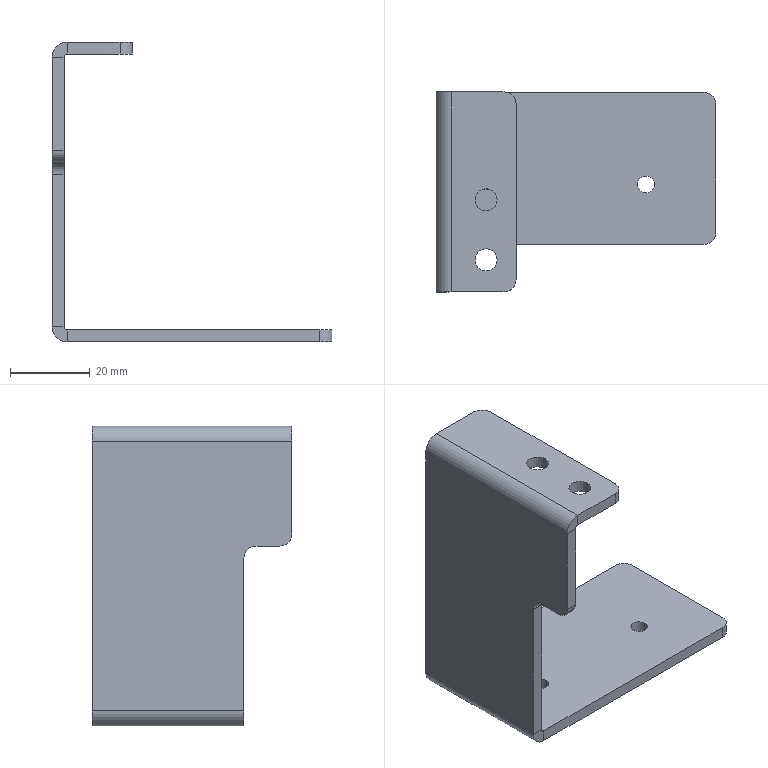Part | SolidWorks | features Fillet 2, HoleWzd 2, FlatPattern 1, ICE 1, SMBaseFlange 1, SheetMetal 1 | 1 solid | 38 faces | box 70 x 50 x 75 mm | volume 19314 mm3 | plane 20 | cylinder 18 | commonest cylinder face diameters 6 x6 4.2 x4 5.5 x4 1.5 x2 7.5 x2
STEP:
#1=CARTESIAN_POINT('',(54.6,27.,-72.));
#2=VERTEX_POINT('',#1);
#3=CARTESIAN_POINT('',(50.4,27.,-72.));
#4=VERTEX_POINT('',#3);
#5=CARTESIAN_POINT('',(52.5,27.,-72.));
#6=DIRECTION('',(0.,0.,-1.));
#7=DIRECTION('',(-1.,0.,0.));
#8=AXIS2_PLACEMENT_3D('',#5,#6,#7);
#9=CIRCLE('',#8,2.1);
#10=EDGE_CURVE('',#2,#4,#9,.T.);
#11=ORIENTED_EDGE('',*,*,#10,.F.);
#12=CARTESIAN_POINT('',(54.6,27.,-75.));
#13=VERTEX_POINT('',#12);
#14=CARTESIAN_POINT('',(54.6,27.,-75.));
#15=DIRECTION('',(0.,0.,-1.));
#16=VECTOR('',#15,1000.);
#17=LINE('',#14,#16);
#18=EDGE_CURVE('',#2,#13,#17,.T.);
#19=ORIENTED_EDGE('',*,*,#18,.T.);
#20=CARTESIAN_POINT('',(50.4,27.,-75.));
#21=VERTEX_POINT('',#20);
#22=CARTESIAN_POINT('',(52.5,27.,-75.));
#23=DIRECTION('',(0.,0.,-1.));
#24=DIRECTION('',(-1.,0.,0.));
#25=AXIS2_PLACEMENT_3D('',#22,#23,#24);
#26=CIRCLE('',#25,2.1);
#27=EDGE_CURVE('',#13,#21,#26,.T.);
#28=ORIENTED_EDGE('',*,*,#27,.T.);
#29=CARTESIAN_POINT('',(50.4,27.,-75.));
#30=DIRECTION('',(0.,0.,-1.));
#31=VECTOR('',#30,1000.);
#32=LINE('',#29,#31);
#33=EDGE_CURVE('',#4,#21,#32,.T.);
#34=ORIENTED_EDGE('',*,*,#33,.F.);
#35=EDGE_LOOP('',(#11,#19,#28,#34));
#36=FACE_OUTER_BOUND('',#35,.T.);
#37=CARTESIAN_POINT('',(52.5,27.,-75.));
#38=DIRECTION('',(0.,0.,-1.));
#39=DIRECTION('',(-1.,0.,0.));
#40=AXIS2_PLACEMENT_3D('',#37,#38,#39);
#41=CYLINDRICAL_SURFACE('',#40,2.1);
#42=ADVANCED_FACE('',(#36),#41,.F.);
#43=CARTESIAN_POINT('',(19.6,27.,-72.));
#44=VERTEX_POINT('',#43);
#45=CARTESIAN_POINT('',(15.4,27.,-72.));
#46=VERTEX_POINT('',#45);
#47=CARTESIAN_POINT('',(17.5,27.,-72.));
#48=DIRECTION('',(0.,0.,-1.));
#49=DIRECTION('',(-1.,0.,0.));
#50=AXIS2_PLACEMENT_3D('',#47,#48,#49);
#51=CIRCLE('',#50,2.1);
#52=EDGE_CURVE('',#44,#46,#51,.T.);
#53=ORIENTED_EDGE('',*,*,#52,.F.);
#54=CARTESIAN_POINT('',(19.6,27.,-75.));
#55=VERTEX_POINT('',#54);
#56=CARTESIAN_POINT('',(19.6,27.,-75.));
#57=DIRECTION('',(0.,0.,-1.));
#58=VECTOR('',#57,1000.);
#59=LINE('',#56,#58);
#60=EDGE_CURVE('',#44,#55,#59,.T.);
#61=ORIENTED_EDGE('',*,*,#60,.T.);
#62=CARTESIAN_POINT('',(15.4,27.,-75.));
#63=VERTEX_POINT('',#62);
#64=CARTESIAN_POINT('',(17.5,27.,-75.));
#65=DIRECTION('',(0.,0.,-1.));
#66=DIRECTION('',(-1.,0.,0.));
#67=AXIS2_PLACEMENT_3D('',#64,#65,#66);
#68=CIRCLE('',#67,2.1);
#69=EDGE_CURVE('',#55,#63,#68,.T.);
#70=ORIENTED_EDGE('',*,*,#69,.T.);
#71=CARTESIAN_POINT('',(15.4,27.,-75.));
#72=DIRECTION('',(0.,0.,-1.));
#73=VECTOR('',#72,1000.);
#74=LINE('',#71,#73);
#75=EDGE_CURVE('',#46,#63,#74,.T.);
#76=ORIENTED_EDGE('',*,*,#75,.F.);
#77=EDGE_LOOP('',(#53,#61,#70,#76));
#78=FACE_OUTER_BOUND('',#77,.T.);
#79=CARTESIAN_POINT('',(17.5,27.,-75.));
#80=DIRECTION('',(0.,0.,-1.));
#81=DIRECTION('',(-1.,0.,0.));
#82=AXIS2_PLACEMENT_3D('',#79,#80,#81);
#83=CYLINDRICAL_SURFACE('',#82,2.1);
#84=ADVANCED_FACE('',(#78),#83,.F.);
#85=CARTESIAN_POINT('',(9.75,23.,-3.));
#86=VERTEX_POINT('',#85);
#87=CARTESIAN_POINT('',(15.25,23.,-3.));
#88=VERTEX_POINT('',#87);
#89=CARTESIAN_POINT('',(12.5,23.,-3.));
#90=DIRECTION('',(0.,0.,1.));
#91=DIRECTION('',(1.,0.,0.));
#92=AXIS2_PLACEMENT_3D('',#89,#90,#91);
#93=CIRCLE('',#92,2.75);
#94=EDGE_CURVE('',#86,#88,#93,.T.);
#95=ORIENTED_EDGE('',*,*,#94,.F.);
#96=CARTESIAN_POINT('',(9.75,23.,0.));
#97=VERTEX_POINT('',#96);
#98=CARTESIAN_POINT('',(9.75,23.,0.));
#99=DIRECTION('',(0.,0.,1.));
#100=VECTOR('',#99,1000.);
#101=LINE('',#98,#100);
#102=EDGE_CURVE('',#86,#97,#101,.T.);
#103=ORIENTED_EDGE('',*,*,#102,.T.);
#104=CARTESIAN_POINT('',(15.25,23.,0.));
#105=VERTEX_POINT('',#104);
#106=CARTESIAN_POINT('',(12.5,23.,0.));
#107=DIRECTION('',(0.,0.,1.));
#108=DIRECTION('',(1.,0.,0.));
#109=AXIS2_PLACEMENT_3D('',#106,#107,#108);
#110=CIRCLE('',#109,2.75);
#111=EDGE_CURVE('',#97,#105,#110,.T.);
#112=ORIENTED_EDGE('',*,*,#111,.T.);
#113=CARTESIAN_POINT('',(15.25,23.,0.));
#114=DIRECTION('',(0.,0.,1.));
#115=VECTOR('',#114,1000.);
#116=LINE('',#113,#115);
#117=EDGE_CURVE('',#88,#105,#116,.T.);
#118=ORIENTED_EDGE('',*,*,#117,.F.);
#119=EDGE_LOOP('',(#95,#103,#112,#118));
#120=FACE_OUTER_BOUND('',#119,.T.);
#121=CARTESIAN_POINT('',(12.5,23.,0.));
#122=DIRECTION('',(0.,0.,1.));
#123=DIRECTION('',(1.,0.,0.));
#124=AXIS2_PLACEMENT_3D('',#121,#122,#123);
#125=CYLINDRICAL_SURFACE('',#124,2.75);
#126=ADVANCED_FACE('',(#120),#125,.F.);
#127=CARTESIAN_POINT('',(9.75,8.,-3.));
#128=VERTEX_POINT('',#127);
#129=CARTESIAN_POINT('',(15.25,8.,-3.));
#130=VERTEX_POINT('',#129);
#131=CARTESIAN_POINT('',(12.5,8.,-3.));
#132=DIRECTION('',(0.,0.,1.));
#133=DIRECTION('',(1.,0.,0.));
#134=AXIS2_PLACEMENT_3D('',#131,#132,#133);
#135=CIRCLE('',#134,2.75);
#136=EDGE_CURVE('',#128,#130,#135,.T.);
#137=ORIENTED_EDGE('',*,*,#136,.F.);
#138=CARTESIAN_POINT('',(9.75,8.,0.));
#139=VERTEX_POINT('',#138);
#140=CARTESIAN_POINT('',(9.75,8.,0.));
#141=DIRECTION('',(0.,0.,1.));
#142=VECTOR('',#141,1000.);
#143=LINE('',#140,#142);
#144=EDGE_CURVE('',#128,#139,#143,.T.);
#145=ORIENTED_EDGE('',*,*,#144,.T.);
#146=CARTESIAN_POINT('',(15.25,8.,0.));
#147=VERTEX_POINT('',#146);
#148=CARTESIAN_POINT('',(12.5,8.,0.));
#149=DIRECTION('',(0.,0.,1.));
#150=DIRECTION('',(1.,0.,0.));
#151=AXIS2_PLACEMENT_3D('',#148,#149,#150);
#152=CIRCLE('',#151,2.75);
#153=EDGE_CURVE('',#139,#147,#152,.T.);
#154=ORIENTED_EDGE('',*,*,#153,.T.);
#155=CARTESIAN_POINT('',(15.25,8.,0.));
#156=DIRECTION('',(0.,0.,1.));
#157=VECTOR('',#156,1000.);
#158=LINE('',#155,#157);
#159=EDGE_CURVE('',#130,#147,#158,.T.);
#160=ORIENTED_EDGE('',*,*,#159,.F.);
#161=EDGE_LOOP('',(#137,#145,#154,#160));
#162=FACE_OUTER_BOUND('',#161,.T.);
#163=CARTESIAN_POINT('',(12.5,8.,0.));
#164=DIRECTION('',(0.,0.,1.));
#165=DIRECTION('',(1.,0.,0.));
#166=AXIS2_PLACEMENT_3D('',#163,#164,#165);
#167=CYLINDRICAL_SURFACE('',#166,2.75);
#168=ADVANCED_FACE('',(#162),#167,.F.);
#169=CARTESIAN_POINT('',(67.,12.,-75.));
#170=VERTEX_POINT('',#169);
#171=CARTESIAN_POINT('',(3.75,12.,-75.));
#172=VERTEX_POINT('',#171);
#173=CARTESIAN_POINT('',(70.,12.,-75.));
#174=DIRECTION('',(-1.,0.,0.));
#175=VECTOR('',#174,1000.);
#176=LINE('',#173,#175);
#177=EDGE_CURVE('',#170,#172,#176,.T.);
#178=ORIENTED_EDGE('',*,*,#177,.F.);
#179=CARTESIAN_POINT('',(67.,12.,-72.));
#180=VERTEX_POINT('',#179);
#181=CARTESIAN_POINT('',(67.,12.,-72.));
#182=DIRECTION('',(0.,0.,1.));
#183=VECTOR('',#182,1000.);
#184=LINE('',#181,#183);
#185=EDGE_CURVE('',#170,#180,#184,.T.);
#186=ORIENTED_EDGE('',*,*,#185,.T.);
#187=CARTESIAN_POINT('',(3.75,12.,-72.));
#188=VERTEX_POINT('',#187);
#189=CARTESIAN_POINT('',(0.,12.,-72.));
#190=DIRECTION('',(1.,0.,0.));
#191=VECTOR('',#190,1000.);
#192=LINE('',#189,#191);
#193=EDGE_CURVE('',#188,#180,#192,.T.);
#194=ORIENTED_EDGE('',*,*,#193,.F.);
#195=CARTESIAN_POINT('',(3.75,12.,-72.));
#196=DIRECTION('',(0.,0.,-1.));
#197=VECTOR('',#196,1000.);
#198=LINE('',#195,#197);
#199=EDGE_CURVE('',#188,#172,#198,.T.);
#200=ORIENTED_EDGE('',*,*,#199,.T.);
#201=EDGE_LOOP('',(#178,#186,#194,#200));
#202=FACE_OUTER_BOUND('',#201,.T.);
#203=CARTESIAN_POINT('',(70.,12.,-75.));
#204=DIRECTION('',(0.,1.,0.));
#205=DIRECTION('',(0.,0.,1.));
#206=AXIS2_PLACEMENT_3D('',#203,#204,#205);
#207=PLANE('',#206);
#208=ADVANCED_FACE('',(#202),#207,.F.);
#209=CARTESIAN_POINT('',(3.,12.,-33.));
#210=VERTEX_POINT('',#209);
#211=CARTESIAN_POINT('',(3.,12.,-71.25));
#212=VERTEX_POINT('',#211);
#213=CARTESIAN_POINT('',(3.,12.,0.));
#214=DIRECTION('',(0.,0.,-1.));
#215=VECTOR('',#214,1000.);
#216=LINE('',#213,#215);
#217=EDGE_CURVE('',#210,#212,#216,.T.);
#218=ORIENTED_EDGE('',*,*,#217,.F.);
#219=CARTESIAN_POINT('',(0.,12.,-33.));
#220=VERTEX_POINT('',#219);
#221=CARTESIAN_POINT('',(0.,12.,-33.));
#222=DIRECTION('',(-1.,0.,0.));
#223=VECTOR('',#222,1000.);
#224=LINE('',#221,#223);
#225=EDGE_CURVE('',#210,#220,#224,.T.);
#226=ORIENTED_EDGE('',*,*,#225,.T.);
#227=CARTESIAN_POINT('',(0.,12.,-71.25));
#228=VERTEX_POINT('',#227);
#229=CARTESIAN_POINT('',(0.,12.,-75.));
#230=DIRECTION('',(0.,0.,-1.));
#231=VECTOR('',#230,1000.);
#232=LINE('',#229,#231);
#233=EDGE_CURVE('',#220,#228,#232,.T.);
#234=ORIENTED_EDGE('',*,*,#233,.T.);
#235=CARTESIAN_POINT('',(0.,12.,-71.25));
#236=DIRECTION('',(1.,0.,0.));
#237=VECTOR('',#236,1000.);
#238=LINE('',#235,#237);
#239=EDGE_CURVE('',#228,#212,#238,.T.);
#240=ORIENTED_EDGE('',*,*,#239,.T.);
#241=EDGE_LOOP('',(#218,#226,#234,#240));
#242=FACE_OUTER_BOUND('',#241,.T.);
#243=CARTESIAN_POINT('',(70.,12.,-75.));
#244=DIRECTION('',(0.,1.,0.));
#245=DIRECTION('',(0.,0.,1.));
#246=AXIS2_PLACEMENT_3D('',#243,#244,#245);
#247=PLANE('',#246);
#248=ADVANCED_FACE('',(#242),#247,.F.);
#249=CARTESIAN_POINT('',(0.,50.,-3.75));
#250=VERTEX_POINT('',#249);
#251=CARTESIAN_POINT('',(3.,50.,-3.75));
#252=VERTEX_POINT('',#251);
#253=CARTESIAN_POINT('',(0.,50.,-3.75));
#254=DIRECTION('',(1.,0.,0.));
#255=VECTOR('',#254,1000.);
#256=LINE('',#253,#255);
#257=EDGE_CURVE('',#250,#252,#256,.T.);
#258=ORIENTED_EDGE('',*,*,#257,.F.);
#259=CARTESIAN_POINT('',(3.75,50.,0.));
#260=VERTEX_POINT('',#259);
#261=CARTESIAN_POINT('',(3.75,50.,-3.75));
#262=DIRECTION('',(0.,-1.,0.));
#263=DIRECTION('',(0.,0.,1.));
#264=AXIS2_PLACEMENT_3D('',#261,#262,#263);
#265=CIRCLE('',#264,3.75);
#266=EDGE_CURVE('',#260,#250,#265,.T.);
#267=ORIENTED_EDGE('',*,*,#266,.F.);
#268=CARTESIAN_POINT('',(3.75,50.,-3.));
#269=VERTEX_POINT('',#268);
#270=CARTESIAN_POINT('',(3.75,50.,-3.));
#271=DIRECTION('',(0.,0.,1.));
#272=VECTOR('',#271,1000.);
#273=LINE('',#270,#272);
#274=EDGE_CURVE('',#269,#260,#273,.T.);
#275=ORIENTED_EDGE('',*,*,#274,.F.);
#276=CARTESIAN_POINT('',(3.75,50.,-3.75));
#277=DIRECTION('',(0.,-1.,0.));
#278=DIRECTION('',(1.,0.,0.));
#279=AXIS2_PLACEMENT_3D('',#276,#277,#278);
#280=CIRCLE('',#279,0.75);
#281=EDGE_CURVE('',#269,#252,#280,.T.);
#282=ORIENTED_EDGE('',*,*,#281,.T.);
#283=EDGE_LOOP('',(#258,#267,#275,#282));
#284=FACE_OUTER_BOUND('',#283,.T.);
#285=CARTESIAN_POINT('',(0.,50.,-3.75));
#286=DIRECTION('',(0.,1.,0.));
#287=DIRECTION('',(0.,0.,1.));
#288=AXIS2_PLACEMENT_3D('',#285,#286,#287);
#289=PLANE('',#288);
#290=ADVANCED_FACE('',(#284),#289,.T.);
#291=CARTESIAN_POINT('',(0.,50.,-71.25));
#292=VERTEX_POINT('',#291);
#293=CARTESIAN_POINT('',(0.,50.,0.));
#294=DIRECTION('',(0.,0.,-1.));
#295=VECTOR('',#294,1000.);
#296=LINE('',#293,#295);
#297=EDGE_CURVE('',#250,#292,#296,.T.);
#298=ORIENTED_EDGE('',*,*,#297,.F.);
#299=ORIENTED_EDGE('',*,*,#257,.T.);
#300=CARTESIAN_POINT('',(3.,50.,-71.25));
#301=VERTEX_POINT('',#300);
#302=CARTESIAN_POINT('',(3.,50.,0.));
#303=DIRECTION('',(0.,0.,-1.));
#304=VECTOR('',#303,1000.);
#305=LINE('',#302,#304);
#306=EDGE_CURVE('',#252,#301,#305,.T.);
#307=ORIENTED_EDGE('',*,*,#306,.T.);
#308=CARTESIAN_POINT('',(3.,50.,-71.25));
#309=DIRECTION('',(-1.,0.,0.));
#310=VECTOR('',#309,1000.);
#311=LINE('',#308,#310);
#312=EDGE_CURVE('',#301,#292,#311,.T.);
#313=ORIENTED_EDGE('',*,*,#312,.T.);
#314=EDGE_LOOP('',(#298,#299,#307,#313));
#315=FACE_OUTER_BOUND('',#314,.T.);
#316=CARTESIAN_POINT('',(3.75,50.,-3.));
#317=DIRECTION('',(0.,1.,0.));
#318=DIRECTION('',(0.,0.,1.));
#319=AXIS2_PLACEMENT_3D('',#316,#317,#318);
#320=PLANE('',#319);
#321=ADVANCED_FACE('',(#315),#320,.T.);
#322=CARTESIAN_POINT('',(3.75,0.,0.));
#323=VERTEX_POINT('',#322);
#324=CARTESIAN_POINT('',(3.75,0.,-3.));
#325=VERTEX_POINT('',#324);
#326=CARTESIAN_POINT('',(3.75,0.,0.));
#327=DIRECTION('',(0.,0.,-1.));
#328=VECTOR('',#327,1000.);
#329=LINE('',#326,#328);
#330=EDGE_CURVE('',#323,#325,#329,.T.);
#331=ORIENTED_EDGE('',*,*,#330,.F.);
#332=CARTESIAN_POINT('',(0.,0.,-3.75));
#333=VERTEX_POINT('',#332);
#334=CARTESIAN_POINT('',(3.75,0.,-3.75));
#335=DIRECTION('',(0.,-1.,0.));
#336=DIRECTION('',(0.,0.,1.));
#337=AXIS2_PLACEMENT_3D('',#334,#335,#336);
#338=CIRCLE('',#337,3.75);
#339=EDGE_CURVE('',#323,#333,#338,.T.);
#340=ORIENTED_EDGE('',*,*,#339,.T.);
#341=CARTESIAN_POINT('',(3.,0.,-3.75));
#342=VERTEX_POINT('',#341);
#343=CARTESIAN_POINT('',(3.,0.,-3.75));
#344=DIRECTION('',(-1.,0.,0.));
#345=VECTOR('',#344,1000.);
#346=LINE('',#343,#345);
#347=EDGE_CURVE('',#342,#333,#346,.T.);
#348=ORIENTED_EDGE('',*,*,#347,.F.);
#349=CARTESIAN_POINT('',(3.75,0.,-3.75));
#350=DIRECTION('',(0.,-1.,0.));
#351=DIRECTION('',(1.,0.,0.));
#352=AXIS2_PLACEMENT_3D('',#349,#350,#351);
#353=CIRCLE('',#352,0.75);
#354=EDGE_CURVE('',#325,#342,#353,.T.);
#355=ORIENTED_EDGE('',*,*,#354,.F.);
#356=EDGE_LOOP('',(#331,#340,#348,#355));
#357=FACE_OUTER_BOUND('',#356,.T.);
#358=CARTESIAN_POINT('',(3.75,0.,0.));
#359=DIRECTION('',(0.,-1.,0.));
#360=DIRECTION('',(0.,0.,-1.));
#361=AXIS2_PLACEMENT_3D('',#358,#359,#360);
#362=PLANE('',#361);
#363=ADVANCED_FACE('',(#357),#362,.T.);
#364=CARTESIAN_POINT('',(17.,0.,-3.));
#365=VERTEX_POINT('',#364);
#366=CARTESIAN_POINT('',(20.,0.,-3.));
#367=DIRECTION('',(-1.,0.,0.));
#368=VECTOR('',#367,1000.);
#369=LINE('',#366,#368);
#370=EDGE_CURVE('',#365,#325,#369,.T.);
#371=ORIENTED_EDGE('',*,*,#370,.F.);
#372=CARTESIAN_POINT('',(17.,0.,0.));
#373=VERTEX_POINT('',#372);
#374=CARTESIAN_POINT('',(17.,0.,-3.75));
#375=DIRECTION('',(0.,0.,1.));
#376=VECTOR('',#375,1000.);
#377=LINE('',#374,#376);
#378=EDGE_CURVE('',#365,#373,#377,.T.);
#379=ORIENTED_EDGE('',*,*,#378,.T.);
#380=CARTESIAN_POINT('',(20.,0.,0.));
#381=DIRECTION('',(-1.,0.,0.));
#382=VECTOR('',#381,1000.);
#383=LINE('',#380,#382);
#384=EDGE_CURVE('',#373,#323,#383,.T.);
#385=ORIENTED_EDGE('',*,*,#384,.T.);
#386=ORIENTED_EDGE('',*,*,#330,.T.);
#387=EDGE_LOOP('',(#371,#379,#385,#386));
#388=FACE_OUTER_BOUND('',#387,.T.);
#389=CARTESIAN_POINT('',(3.,0.,-3.75));
#390=DIRECTION('',(0.,-1.,0.));
#391=DIRECTION('',(0.,0.,-1.));
#392=AXIS2_PLACEMENT_3D('',#389,#390,#391);
#393=PLANE('',#392);
#394=ADVANCED_FACE('',(#388),#393,.T.);
#395=CARTESIAN_POINT('',(3.75,50.,-75.));
#396=VERTEX_POINT('',#395);
#397=CARTESIAN_POINT('',(3.75,50.,-72.));
#398=VERTEX_POINT('',#397);
#399=CARTESIAN_POINT('',(3.75,50.,-75.));
#400=DIRECTION('',(0.,0.,1.));
#401=VECTOR('',#400,1000.);
#402=LINE('',#399,#401);
#403=EDGE_CURVE('',#396,#398,#402,.T.);
#404=ORIENTED_EDGE('',*,*,#403,.F.);
#405=CARTESIAN_POINT('',(3.75,50.,-71.25));
#406=DIRECTION('',(0.,-1.,0.));
#407=DIRECTION('',(0.,0.,1.));
#408=AXIS2_PLACEMENT_3D('',#405,#406,#407);
#409=CIRCLE('',#408,3.75);
#410=EDGE_CURVE('',#292,#396,#409,.T.);
#411=ORIENTED_EDGE('',*,*,#410,.F.);
#412=ORIENTED_EDGE('',*,*,#312,.F.);
#413=CARTESIAN_POINT('',(3.75,50.,-71.25));
#414=DIRECTION('',(0.,-1.,0.));
#415=DIRECTION('',(1.,0.,0.));
#416=AXIS2_PLACEMENT_3D('',#413,#414,#415);
#417=CIRCLE('',#416,0.75);
#418=EDGE_CURVE('',#301,#398,#417,.T.);
#419=ORIENTED_EDGE('',*,*,#418,.T.);
#420=EDGE_LOOP('',(#404,#411,#412,#419));
#421=FACE_OUTER_BOUND('',#420,.T.);
#422=CARTESIAN_POINT('',(3.75,50.,-75.));
#423=DIRECTION('',(0.,1.,0.));
#424=DIRECTION('',(0.,0.,1.));
#425=AXIS2_PLACEMENT_3D('',#422,#423,#424);
#426=PLANE('',#425);
#427=ADVANCED_FACE('',(#421),#426,.T.);
#428=CARTESIAN_POINT('',(67.,50.,-72.));
#429=VERTEX_POINT('',#428);
#430=CARTESIAN_POINT('',(0.,50.,-72.));
#431=DIRECTION('',(1.,0.,0.));
#432=VECTOR('',#431,1000.);
#433=LINE('',#430,#432);
#434=EDGE_CURVE('',#398,#429,#433,.T.);
#435=ORIENTED_EDGE('',*,*,#434,.T.);
#436=CARTESIAN_POINT('',(67.,50.,-75.));
#437=VERTEX_POINT('',#436);
#438=CARTESIAN_POINT('',(67.,50.,-71.25));
#439=DIRECTION('',(0.,0.,-1.));
#440=VECTOR('',#439,1000.);
#441=LINE('',#438,#440);
#442=EDGE_CURVE('',#429,#437,#441,.T.);
#443=ORIENTED_EDGE('',*,*,#442,.T.);
#444=CARTESIAN_POINT('',(0.,50.,-75.));
#445=DIRECTION('',(1.,0.,0.));
#446=VECTOR('',#445,1000.);
#447=LINE('',#444,#446);
#448=EDGE_CURVE('',#396,#437,#447,.T.);
#449=ORIENTED_EDGE('',*,*,#448,.F.);
#450=ORIENTED_EDGE('',*,*,#403,.T.);
#451=EDGE_LOOP('',(#435,#443,#449,#450));
#452=FACE_OUTER_BOUND('',#451,.T.);
#453=CARTESIAN_POINT('',(3.,50.,-71.25));
#454=DIRECTION('',(0.,1.,0.));
#455=DIRECTION('',(0.,0.,1.));
#456=AXIS2_PLACEMENT_3D('',#453,#454,#455);
#457=PLANE('',#456);
#458=ADVANCED_FACE('',(#452),#457,.T.);
#459=CARTESIAN_POINT('',(0.,0.,-27.));
#460=VERTEX_POINT('',#459);
#461=CARTESIAN_POINT('',(0.,0.,0.));
#462=DIRECTION('',(0.,0.,-1.));
#463=VECTOR('',#462,1000.);
#464=LINE('',#461,#463);
#465=EDGE_CURVE('',#333,#460,#464,.T.);
#466=ORIENTED_EDGE('',*,*,#465,.T.);
#467=CARTESIAN_POINT('',(3.,0.,-27.));
#468=VERTEX_POINT('',#467);
#469=CARTESIAN_POINT('',(3.,0.,-27.));
#470=DIRECTION('',(1.,0.,0.));
#471=VECTOR('',#470,1000.);
#472=LINE('',#469,#471);
#473=EDGE_CURVE('',#460,#468,#472,.T.);
#474=ORIENTED_EDGE('',*,*,#473,.T.);
#475=CARTESIAN_POINT('',(3.,0.,0.));
#476=DIRECTION('',(0.,0.,-1.));
#477=VECTOR('',#476,1000.);
#478=LINE('',#475,#477);
#479=EDGE_CURVE('',#342,#468,#478,.T.);
#480=ORIENTED_EDGE('',*,*,#479,.F.);
#481=ORIENTED_EDGE('',*,*,#347,.T.);
#482=EDGE_LOOP('',(#466,#474,#480,#481));
#483=FACE_OUTER_BOUND('',#482,.T.);
#484=CARTESIAN_POINT('',(3.75,0.,-72.));
#485=DIRECTION('',(0.,-1.,0.));
#486=DIRECTION('',(0.,0.,-1.));
#487=AXIS2_PLACEMENT_3D('',#484,#485,#486);
#488=PLANE('',#487);
#489=ADVANCED_FACE('',(#483),#488,.T.);
#490=CARTESIAN_POINT('',(52.5,27.,-72.));
#491=DIRECTION('',(0.,0.,-1.));
#492=DIRECTION('',(-1.,0.,0.));
#493=AXIS2_PLACEMENT_3D('',#490,#491,#492);
#494=CIRCLE('',#493,2.1);
#495=EDGE_CURVE('',#4,#2,#494,.T.);
#496=ORIENTED_EDGE('',*,*,#495,.T.);
#497=ORIENTED_EDGE('',*,*,#10,.T.);
#498=EDGE_LOOP('',(#496,#497));
#499=FACE_BOUND('',#498,.T.);
#500=CARTESIAN_POINT('',(17.5,27.,-72.));
#501=DIRECTION('',(0.,0.,-1.));
#502=DIRECTION('',(-1.,0.,0.));
#503=AXIS2_PLACEMENT_3D('',#500,#501,#502);
#504=CIRCLE('',#503,2.1);
#505=EDGE_CURVE('',#46,#44,#504,.T.);
#506=ORIENTED_EDGE('',*,*,#505,.T.);
#507=ORIENTED_EDGE('',*,*,#52,.T.);
#508=EDGE_LOOP('',(#506,#507));
#509=FACE_BOUND('',#508,.T.);
#510=ORIENTED_EDGE('',*,*,#193,.T.);
#511=CARTESIAN_POINT('',(70.,15.,-72.));
#512=VERTEX_POINT('',#511);
#513=CARTESIAN_POINT('',(67.,15.,-72.));
#514=DIRECTION('',(0.,0.,1.));
#515=DIRECTION('',(-1.,0.,0.));
#516=AXIS2_PLACEMENT_3D('',#513,#514,#515);
#517=CIRCLE('',#516,3.);
#518=EDGE_CURVE('',#180,#512,#517,.T.);
#519=ORIENTED_EDGE('',*,*,#518,.T.);
#520=CARTESIAN_POINT('',(70.,47.,-72.));
#521=VERTEX_POINT('',#520);
#522=CARTESIAN_POINT('',(70.,50.,-72.));
#523=DIRECTION('',(0.,-1.,0.));
#524=VECTOR('',#523,1000.);
#525=LINE('',#522,#524);
#526=EDGE_CURVE('',#521,#512,#525,.T.);
#527=ORIENTED_EDGE('',*,*,#526,.F.);
#528=CARTESIAN_POINT('',(67.,47.,-72.));
#529=DIRECTION('',(0.,0.,1.));
#530=DIRECTION('',(-1.,0.,0.));
#531=AXIS2_PLACEMENT_3D('',#528,#529,#530);
#532=CIRCLE('',#531,3.);
#533=EDGE_CURVE('',#521,#429,#532,.T.);
#534=ORIENTED_EDGE('',*,*,#533,.T.);
#535=ORIENTED_EDGE('',*,*,#434,.F.);
#536=CARTESIAN_POINT('',(3.75,50.,-72.));
#537=DIRECTION('',(0.,-1.,0.));
#538=VECTOR('',#537,1000.);
#539=LINE('',#536,#538);
#540=EDGE_CURVE('',#398,#188,#539,.T.);
#541=ORIENTED_EDGE('',*,*,#540,.T.);
#542=EDGE_LOOP('',(#510,#519,#527,#534,#535,#541));
#543=FACE_OUTER_BOUND('',#542,.T.);
#544=CARTESIAN_POINT('',(0.,50.,-72.));
#545=DIRECTION('',(0.,0.,-1.));
#546=DIRECTION('',(-1.,0.,0.));
#547=AXIS2_PLACEMENT_3D('',#544,#545,#546);
#548=PLANE('',#547);
#549=ADVANCED_FACE('',(#499,#509,#543),#548,.F.);
#550=ORIENTED_EDGE('',*,*,#526,.T.);
#551=CARTESIAN_POINT('',(70.,15.,-75.));
#552=VERTEX_POINT('',#551);
#553=CARTESIAN_POINT('',(70.,15.,-75.));
#554=DIRECTION('',(0.,0.,-1.));
#555=VECTOR('',#554,1000.);
#556=LINE('',#553,#555);
#557=EDGE_CURVE('',#512,#552,#556,.T.);
#558=ORIENTED_EDGE('',*,*,#557,.T.);
#559=CARTESIAN_POINT('',(70.,47.,-75.));
#560=VERTEX_POINT('',#559);
#561=CARTESIAN_POINT('',(70.,50.,-75.));
#562=DIRECTION('',(0.,-1.,0.));
#563=VECTOR('',#562,1000.);
#564=LINE('',#561,#563);
#565=EDGE_CURVE('',#560,#552,#564,.T.);
#566=ORIENTED_EDGE('',*,*,#565,.F.);
#567=CARTESIAN_POINT('',(70.,47.,-75.));
#568=DIRECTION('',(0.,0.,1.));
#569=VECTOR('',#568,1000.);
#570=LINE('',#567,#569);
#571=EDGE_CURVE('',#560,#521,#570,.T.);
#572=ORIENTED_EDGE('',*,*,#571,.T.);
#573=EDGE_LOOP('',(#550,#558,#566,#572));
#574=FACE_OUTER_BOUND('',#573,.T.);
#575=CARTESIAN_POINT('',(70.,50.,-75.));
#576=DIRECTION('',(1.,0.,0.));
#577=DIRECTION('',(0.,0.,-1.));
#578=AXIS2_PLACEMENT_3D('',#575,#576,#577);
#579=PLANE('',#578);
#580=ADVANCED_FACE('',(#574),#579,.T.);
#581=CARTESIAN_POINT('',(52.5,27.,-75.));
#582=DIRECTION('',(0.,0.,-1.));
#583=DIRECTION('',(-1.,0.,0.));
#584=AXIS2_PLACEMENT_3D('',#581,#582,#583);
#585=CIRCLE('',#584,2.1);
#586=EDGE_CURVE('',#21,#13,#585,.T.);
#587=ORIENTED_EDGE('',*,*,#586,.F.);
#588=ORIENTED_EDGE('',*,*,#27,.F.);
#589=EDGE_LOOP('',(#587,#588));
#590=FACE_BOUND('',#589,.T.);
#591=CARTESIAN_POINT('',(17.5,27.,-75.));
#592=DIRECTION('',(0.,0.,-1.));
#593=DIRECTION('',(-1.,0.,0.));
#594=AXIS2_PLACEMENT_3D('',#591,#592,#593);
#595=CIRCLE('',#594,2.1);
#596=EDGE_CURVE('',#63,#55,#595,.T.);
#597=ORIENTED_EDGE('',*,*,#596,.F.);
#598=ORIENTED_EDGE('',*,*,#69,.F.);
#599=EDGE_LOOP('',(#597,#598));
#600=FACE_BOUND('',#599,.T.);
#601=ORIENTED_EDGE('',*,*,#565,.T.);
#602=CARTESIAN_POINT('',(67.,15.,-75.));
#603=DIRECTION('',(0.,0.,-1.));
#604=DIRECTION('',(-1.,0.,0.));
#605=AXIS2_PLACEMENT_3D('',#602,#603,#604);
#606=CIRCLE('',#605,3.);
#607=EDGE_CURVE('',#552,#170,#606,.T.);
#608=ORIENTED_EDGE('',*,*,#607,.T.);
#609=ORIENTED_EDGE('',*,*,#177,.T.);
#610=CARTESIAN_POINT('',(3.75,50.,-75.));
#611=DIRECTION('',(0.,-1.,0.));
#612=VECTOR('',#611,1000.);
#613=LINE('',#610,#612);
#614=EDGE_CURVE('',#396,#172,#613,.T.);
#615=ORIENTED_EDGE('',*,*,#614,.F.);
#616=ORIENTED_EDGE('',*,*,#448,.T.);
#617=CARTESIAN_POINT('',(67.,47.,-75.));
#618=DIRECTION('',(0.,0.,-1.));
#619=DIRECTION('',(-1.,0.,0.));
#620=AXIS2_PLACEMENT_3D('',#617,#618,#619);
#621=CIRCLE('',#620,3.);
#622=EDGE_CURVE('',#437,#560,#621,.T.);
#623=ORIENTED_EDGE('',*,*,#622,.T.);
#624=EDGE_LOOP('',(#601,#608,#609,#615,#616,#623));
#625=FACE_OUTER_BOUND('',#624,.T.);
#626=CARTESIAN_POINT('',(0.,50.,-75.));
#627=DIRECTION('',(0.,0.,-1.));
#628=DIRECTION('',(-1.,0.,0.));
#629=AXIS2_PLACEMENT_3D('',#626,#627,#628);
#630=PLANE('',#629);
#631=ADVANCED_FACE('',(#590,#600,#625),#630,.T.);
#632=CARTESIAN_POINT('',(3.75,12.,-71.25));
#633=DIRECTION('',(0.,-1.,0.));
#634=DIRECTION('',(0.,0.,1.));
#635=AXIS2_PLACEMENT_3D('',#632,#633,#634);
#636=CIRCLE('',#635,3.75);
#637=EDGE_CURVE('',#228,#172,#636,.T.);
#638=ORIENTED_EDGE('',*,*,#637,.F.);
#639=CARTESIAN_POINT('',(0.,50.,-71.25));
#640=DIRECTION('',(0.,-1.,0.));
#641=VECTOR('',#640,1000.);
#642=LINE('',#639,#641);
#643=EDGE_CURVE('',#292,#228,#642,.T.);
#644=ORIENTED_EDGE('',*,*,#643,.F.);
#645=ORIENTED_EDGE('',*,*,#410,.T.);
#646=ORIENTED_EDGE('',*,*,#614,.T.);
#647=EDGE_LOOP('',(#638,#644,#645,#646));
#648=FACE_OUTER_BOUND('',#647,.T.);
#649=CARTESIAN_POINT('',(3.75,50.,-71.25));
#650=DIRECTION('',(0.,-1.,0.));
#651=DIRECTION('',(0.,0.,-1.));
#652=AXIS2_PLACEMENT_3D('',#649,#650,#651);
#653=CYLINDRICAL_SURFACE('',#652,3.75);
#654=ADVANCED_FACE('',(#648),#653,.T.);
#655=CARTESIAN_POINT('',(0.,3.,-30.));
#656=VERTEX_POINT('',#655);
#657=CARTESIAN_POINT('',(0.,9.,-30.));
#658=VERTEX_POINT('',#657);
#659=CARTESIAN_POINT('',(0.,0.,-30.));
#660=DIRECTION('',(0.,1.,0.));
#661=VECTOR('',#660,1000.);
#662=LINE('',#659,#661);
#663=EDGE_CURVE('',#656,#658,#662,.T.);
#664=ORIENTED_EDGE('',*,*,#663,.F.);
#665=CARTESIAN_POINT('',(0.,3.,-27.));
#666=DIRECTION('',(-1.,0.,0.));
#667=DIRECTION('',(0.,0.,1.));
#668=AXIS2_PLACEMENT_3D('',#665,#666,#667);
#669=CIRCLE('',#668,3.);
#670=EDGE_CURVE('',#656,#460,#669,.T.);
#671=ORIENTED_EDGE('',*,*,#670,.T.);
#672=ORIENTED_EDGE('',*,*,#465,.F.);
#673=CARTESIAN_POINT('',(0.,50.,-3.75));
#674=DIRECTION('',(0.,-1.,0.));
#675=VECTOR('',#674,1000.);
#676=LINE('',#673,#675);
#677=EDGE_CURVE('',#250,#333,#676,.T.);
#678=ORIENTED_EDGE('',*,*,#677,.F.);
#679=ORIENTED_EDGE('',*,*,#297,.T.);
#680=ORIENTED_EDGE('',*,*,#643,.T.);
#681=ORIENTED_EDGE('',*,*,#233,.F.);
#682=CARTESIAN_POINT('',(0.,9.,-33.));
#683=DIRECTION('',(1.,0.,0.));
#684=DIRECTION('',(0.,0.,1.));
#685=AXIS2_PLACEMENT_3D('',#682,#683,#684);
#686=CIRCLE('',#685,3.);
#687=EDGE_CURVE('',#220,#658,#686,.T.);
#688=ORIENTED_EDGE('',*,*,#687,.T.);
#689=EDGE_LOOP('',(#664,#671,#672,#678,#679,#680,#681,#688));
#690=FACE_OUTER_BOUND('',#689,.T.);
#691=CARTESIAN_POINT('',(0.,50.,0.));
#692=DIRECTION('',(-1.,0.,0.));
#693=DIRECTION('',(0.,0.,1.));
#694=AXIS2_PLACEMENT_3D('',#691,#692,#693);
#695=PLANE('',#694);
#696=ADVANCED_FACE('',(#690),#695,.T.);
#697=ORIENTED_EDGE('',*,*,#339,.F.);
#698=CARTESIAN_POINT('',(3.75,50.,0.));
#699=DIRECTION('',(0.,-1.,0.));
#700=VECTOR('',#699,1000.);
#701=LINE('',#698,#700);
#702=EDGE_CURVE('',#260,#323,#701,.T.);
#703=ORIENTED_EDGE('',*,*,#702,.F.);
#704=ORIENTED_EDGE('',*,*,#266,.T.);
#705=ORIENTED_EDGE('',*,*,#677,.T.);
#706=EDGE_LOOP('',(#697,#703,#704,#705));
#707=FACE_OUTER_BOUND('',#706,.T.);
#708=CARTESIAN_POINT('',(3.75,50.,-3.75));
#709=DIRECTION('',(0.,-1.,0.));
#710=DIRECTION('',(0.,0.,-1.));
#711=AXIS2_PLACEMENT_3D('',#708,#709,#710);
#712=CYLINDRICAL_SURFACE('',#711,3.75);
#713=ADVANCED_FACE('',(#707),#712,.T.);
#714=CARTESIAN_POINT('',(12.5,23.,0.));
#715=DIRECTION('',(0.,0.,1.));
#716=DIRECTION('',(1.,0.,0.));
#717=AXIS2_PLACEMENT_3D('',#714,#715,#716);
#718=CIRCLE('',#717,2.75);
#719=EDGE_CURVE('',#105,#97,#718,.T.);
#720=ORIENTED_EDGE('',*,*,#719,.F.);
#721=ORIENTED_EDGE('',*,*,#111,.F.);
#722=EDGE_LOOP('',(#720,#721));
#723=FACE_BOUND('',#722,.T.);
#724=CARTESIAN_POINT('',(12.5,8.,0.));
#725=DIRECTION('',(0.,0.,1.));
#726=DIRECTION('',(1.,0.,0.));
#727=AXIS2_PLACEMENT_3D('',#724,#725,#726);
#728=CIRCLE('',#727,2.75);
#729=EDGE_CURVE('',#147,#139,#728,.T.);
#730=ORIENTED_EDGE('',*,*,#729,.F.);
#731=ORIENTED_EDGE('',*,*,#153,.F.);
#732=EDGE_LOOP('',(#730,#731));
#733=FACE_BOUND('',#732,.T.);
#734=ORIENTED_EDGE('',*,*,#384,.F.);
#735=CARTESIAN_POINT('',(20.,3.,0.));
#736=VERTEX_POINT('',#735);
#737=CARTESIAN_POINT('',(17.,3.,0.));
#738=DIRECTION('',(0.,0.,1.));
#739=DIRECTION('',(1.,0.,0.));
#740=AXIS2_PLACEMENT_3D('',#737,#738,#739);
#741=CIRCLE('',#740,3.);
#742=EDGE_CURVE('',#373,#736,#741,.T.);
#743=ORIENTED_EDGE('',*,*,#742,.T.);
#744=CARTESIAN_POINT('',(20.,47.,0.));
#745=VERTEX_POINT('',#744);
#746=CARTESIAN_POINT('',(20.,50.,0.));
#747=DIRECTION('',(0.,-1.,0.));
#748=VECTOR('',#747,1000.);
#749=LINE('',#746,#748);
#750=EDGE_CURVE('',#745,#736,#749,.T.);
#751=ORIENTED_EDGE('',*,*,#750,.F.);
#752=CARTESIAN_POINT('',(17.,50.,0.));
#753=VERTEX_POINT('',#752);
#754=CARTESIAN_POINT('',(17.,47.,0.));
#755=DIRECTION('',(0.,0.,1.));
#756=DIRECTION('',(1.,0.,0.));
#757=AXIS2_PLACEMENT_3D('',#754,#755,#756);
#758=CIRCLE('',#757,3.);
#759=EDGE_CURVE('',#745,#753,#758,.T.);
#760=ORIENTED_EDGE('',*,*,#759,.T.);
#761=CARTESIAN_POINT('',(20.,50.,0.));
#762=DIRECTION('',(-1.,0.,0.));
#763=VECTOR('',#762,1000.);
#764=LINE('',#761,#763);
#765=EDGE_CURVE('',#753,#260,#764,.T.);
#766=ORIENTED_EDGE('',*,*,#765,.T.);
#767=ORIENTED_EDGE('',*,*,#702,.T.);
#768=EDGE_LOOP('',(#734,#743,#751,#760,#766,#767));
#769=FACE_OUTER_BOUND('',#768,.T.);
#770=CARTESIAN_POINT('',(20.,50.,0.));
#771=DIRECTION('',(0.,0.,1.));
#772=DIRECTION('',(1.,0.,0.));
#773=AXIS2_PLACEMENT_3D('',#770,#771,#772);
#774=PLANE('',#773);
#775=ADVANCED_FACE('',(#723,#733,#769),#774,.T.);
#776=ORIENTED_EDGE('',*,*,#750,.T.);
#777=CARTESIAN_POINT('',(20.,3.,-3.));
#778=VERTEX_POINT('',#777);
#779=CARTESIAN_POINT('',(20.,3.,-3.));
#780=DIRECTION('',(0.,0.,-1.));
#781=VECTOR('',#780,1000.);
#782=LINE('',#779,#781);
#783=EDGE_CURVE('',#736,#778,#782,.T.);
#784=ORIENTED_EDGE('',*,*,#783,.T.);
#785=CARTESIAN_POINT('',(20.,47.,-3.));
#786=VERTEX_POINT('',#785);
#787=CARTESIAN_POINT('',(20.,50.,-3.));
#788=DIRECTION('',(0.,-1.,0.));
#789=VECTOR('',#788,1000.);
#790=LINE('',#787,#789);
#791=EDGE_CURVE('',#786,#778,#790,.T.);
#792=ORIENTED_EDGE('',*,*,#791,.F.);
#793=CARTESIAN_POINT('',(20.,47.,-3.));
#794=DIRECTION('',(0.,0.,1.));
#795=VECTOR('',#794,1000.);
#796=LINE('',#793,#795);
#797=EDGE_CURVE('',#786,#745,#796,.T.);
#798=ORIENTED_EDGE('',*,*,#797,.T.);
#799=EDGE_LOOP('',(#776,#784,#792,#798));
#800=FACE_OUTER_BOUND('',#799,.T.);
#801=CARTESIAN_POINT('',(20.,50.,-3.));
#802=DIRECTION('',(1.,0.,0.));
#803=DIRECTION('',(0.,0.,-1.));
#804=AXIS2_PLACEMENT_3D('',#801,#802,#803);
#805=PLANE('',#804);
#806=ADVANCED_FACE('',(#800),#805,.T.);
#807=CARTESIAN_POINT('',(12.5,23.,-3.));
#808=DIRECTION('',(0.,0.,1.));
#809=DIRECTION('',(1.,0.,0.));
#810=AXIS2_PLACEMENT_3D('',#807,#808,#809);
#811=CIRCLE('',#810,2.75);
#812=EDGE_CURVE('',#88,#86,#811,.T.);
#813=ORIENTED_EDGE('',*,*,#812,.T.);
#814=ORIENTED_EDGE('',*,*,#94,.T.);
#815=EDGE_LOOP('',(#813,#814));
#816=FACE_BOUND('',#815,.T.);
#817=CARTESIAN_POINT('',(12.5,8.,-3.));
#818=DIRECTION('',(0.,0.,1.));
#819=DIRECTION('',(1.,0.,0.));
#820=AXIS2_PLACEMENT_3D('',#817,#818,#819);
#821=CIRCLE('',#820,2.75);
#822=EDGE_CURVE('',#130,#128,#821,.T.);
#823=ORIENTED_EDGE('',*,*,#822,.T.);
#824=ORIENTED_EDGE('',*,*,#136,.T.);
#825=EDGE_LOOP('',(#823,#824));
#826=FACE_BOUND('',#825,.T.);
#827=ORIENTED_EDGE('',*,*,#791,.T.);
#828=CARTESIAN_POINT('',(17.,3.,-3.));
#829=DIRECTION('',(0.,0.,-1.));
#830=DIRECTION('',(1.,0.,0.));
#831=AXIS2_PLACEMENT_3D('',#828,#829,#830);
#832=CIRCLE('',#831,3.);
#833=EDGE_CURVE('',#778,#365,#832,.T.);
#834=ORIENTED_EDGE('',*,*,#833,.T.);
#835=ORIENTED_EDGE('',*,*,#370,.T.);
#836=CARTESIAN_POINT('',(3.75,50.,-3.));
#837=DIRECTION('',(0.,-1.,0.));
#838=VECTOR('',#837,1000.);
#839=LINE('',#836,#838);
#840=EDGE_CURVE('',#269,#325,#839,.T.);
#841=ORIENTED_EDGE('',*,*,#840,.F.);
#842=CARTESIAN_POINT('',(17.,50.,-3.));
#843=VERTEX_POINT('',#842);
#844=CARTESIAN_POINT('',(20.,50.,-3.));
#845=DIRECTION('',(-1.,0.,0.));
#846=VECTOR('',#845,1000.);
#847=LINE('',#844,#846);
#848=EDGE_CURVE('',#843,#269,#847,.T.);
#849=ORIENTED_EDGE('',*,*,#848,.F.);
#850=CARTESIAN_POINT('',(17.,47.,-3.));
#851=DIRECTION('',(0.,0.,-1.));
#852=DIRECTION('',(1.,0.,0.));
#853=AXIS2_PLACEMENT_3D('',#850,#851,#852);
#854=CIRCLE('',#853,3.);
#855=EDGE_CURVE('',#843,#786,#854,.T.);
#856=ORIENTED_EDGE('',*,*,#855,.T.);
#857=EDGE_LOOP('',(#827,#834,#835,#841,#849,#856));
#858=FACE_OUTER_BOUND('',#857,.T.);
#859=CARTESIAN_POINT('',(20.,50.,-3.));
#860=DIRECTION('',(0.,0.,1.));
#861=DIRECTION('',(1.,0.,0.));
#862=AXIS2_PLACEMENT_3D('',#859,#860,#861);
#863=PLANE('',#862);
#864=ADVANCED_FACE('',(#816,#826,#858),#863,.F.);
#865=ORIENTED_EDGE('',*,*,#354,.T.);
#866=CARTESIAN_POINT('',(3.,50.,-3.75));
#867=DIRECTION('',(0.,-1.,0.));
#868=VECTOR('',#867,1000.);
#869=LINE('',#866,#868);
#870=EDGE_CURVE('',#252,#342,#869,.T.);
#871=ORIENTED_EDGE('',*,*,#870,.F.);
#872=ORIENTED_EDGE('',*,*,#281,.F.);
#873=ORIENTED_EDGE('',*,*,#840,.T.);
#874=EDGE_LOOP('',(#865,#871,#872,#873));
#875=FACE_OUTER_BOUND('',#874,.T.);
#876=CARTESIAN_POINT('',(3.75,50.,-3.75));
#877=DIRECTION('',(0.,-1.,0.));
#878=DIRECTION('',(0.,0.,-1.));
#879=AXIS2_PLACEMENT_3D('',#876,#877,#878);
#880=CYLINDRICAL_SURFACE('',#879,0.75);
#881=ADVANCED_FACE('',(#875),#880,.F.);
#882=ORIENTED_EDGE('',*,*,#479,.T.);
#883=CARTESIAN_POINT('',(3.,3.,-30.));
#884=VERTEX_POINT('',#883);
#885=CARTESIAN_POINT('',(3.,3.,-27.));
#886=DIRECTION('',(1.,0.,0.));
#887=DIRECTION('',(0.,0.,1.));
#888=AXIS2_PLACEMENT_3D('',#885,#886,#887);
#889=CIRCLE('',#888,3.);
#890=EDGE_CURVE('',#468,#884,#889,.T.);
#891=ORIENTED_EDGE('',*,*,#890,.T.);
#892=CARTESIAN_POINT('',(3.,9.,-30.));
#893=VERTEX_POINT('',#892);
#894=CARTESIAN_POINT('',(3.,50.,-30.));
#895=DIRECTION('',(0.,1.,0.));
#896=VECTOR('',#895,1000.);
#897=LINE('',#894,#896);
#898=EDGE_CURVE('',#884,#893,#897,.T.);
#899=ORIENTED_EDGE('',*,*,#898,.T.);
#900=CARTESIAN_POINT('',(3.,9.,-33.));
#901=DIRECTION('',(-1.,0.,0.));
#902=DIRECTION('',(0.,0.,1.));
#903=AXIS2_PLACEMENT_3D('',#900,#901,#902);
#904=CIRCLE('',#903,3.);
#905=EDGE_CURVE('',#893,#210,#904,.T.);
#906=ORIENTED_EDGE('',*,*,#905,.T.);
#907=ORIENTED_EDGE('',*,*,#217,.T.);
#908=CARTESIAN_POINT('',(3.,50.,-71.25));
#909=DIRECTION('',(0.,-1.,0.));
#910=VECTOR('',#909,1000.);
#911=LINE('',#908,#910);
#912=EDGE_CURVE('',#301,#212,#911,.T.);
#913=ORIENTED_EDGE('',*,*,#912,.F.);
#914=ORIENTED_EDGE('',*,*,#306,.F.);
#915=ORIENTED_EDGE('',*,*,#870,.T.);
#916=EDGE_LOOP('',(#882,#891,#899,#906,#907,#913,#914,#915));
#917=FACE_OUTER_BOUND('',#916,.T.);
#918=CARTESIAN_POINT('',(3.,50.,0.));
#919=DIRECTION('',(-1.,0.,0.));
#920=DIRECTION('',(0.,0.,1.));
#921=AXIS2_PLACEMENT_3D('',#918,#919,#920);
#922=PLANE('',#921);
#923=ADVANCED_FACE('',(#917),#922,.F.);
#924=ORIENTED_EDGE('',*,*,#912,.T.);
#925=CARTESIAN_POINT('',(3.75,12.,-71.25));
#926=DIRECTION('',(0.,-1.,0.));
#927=DIRECTION('',(0.,0.,1.));
#928=AXIS2_PLACEMENT_3D('',#925,#926,#927);
#929=CIRCLE('',#928,0.75);
#930=EDGE_CURVE('',#212,#188,#929,.T.);
#931=ORIENTED_EDGE('',*,*,#930,.T.);
#932=ORIENTED_EDGE('',*,*,#540,.F.);
#933=ORIENTED_EDGE('',*,*,#418,.F.);
#934=EDGE_LOOP('',(#924,#931,#932,#933));
#935=FACE_OUTER_BOUND('',#934,.T.);
#936=CARTESIAN_POINT('',(3.75,50.,-71.25));
#937=DIRECTION('',(0.,-1.,0.));
#938=DIRECTION('',(0.,0.,-1.));
#939=AXIS2_PLACEMENT_3D('',#936,#937,#938);
#940=CYLINDRICAL_SURFACE('',#939,0.75);
#941=ADVANCED_FACE('',(#935),#940,.F.);
#942=ORIENTED_EDGE('',*,*,#765,.F.);
#943=CARTESIAN_POINT('',(17.,50.,-71.25));
#944=DIRECTION('',(0.,0.,-1.));
#945=VECTOR('',#944,1000.);
#946=LINE('',#943,#945);
#947=EDGE_CURVE('',#753,#843,#946,.T.);
#948=ORIENTED_EDGE('',*,*,#947,.T.);
#949=ORIENTED_EDGE('',*,*,#848,.T.);
#950=ORIENTED_EDGE('',*,*,#274,.T.);
#951=EDGE_LOOP('',(#942,#948,#949,#950));
#952=FACE_OUTER_BOUND('',#951,.T.);
#953=CARTESIAN_POINT('',(3.75,50.,-71.25));
#954=DIRECTION('',(0.,1.,0.));
#955=DIRECTION('',(1.,0.,0.));
#956=AXIS2_PLACEMENT_3D('',#953,#954,#955);
#957=PLANE('',#956);
#958=ADVANCED_FACE('',(#952),#957,.T.);
#959=ORIENTED_EDGE('',*,*,#833,.F.);
#960=ORIENTED_EDGE('',*,*,#783,.F.);
#961=ORIENTED_EDGE('',*,*,#742,.F.);
#962=ORIENTED_EDGE('',*,*,#378,.F.);
#963=EDGE_LOOP('',(#959,#960,#961,#962));
#964=FACE_OUTER_BOUND('',#963,.T.);
#965=CARTESIAN_POINT('',(17.,3.,-3.75));
#966=DIRECTION('',(0.,0.,1.));
#967=DIRECTION('',(1.,0.,0.));
#968=AXIS2_PLACEMENT_3D('',#965,#966,#967);
#969=CYLINDRICAL_SURFACE('',#968,3.);
#970=ADVANCED_FACE('',(#964),#969,.T.);
#971=ORIENTED_EDGE('',*,*,#855,.F.);
#972=ORIENTED_EDGE('',*,*,#947,.F.);
#973=ORIENTED_EDGE('',*,*,#759,.F.);
#974=ORIENTED_EDGE('',*,*,#797,.F.);
#975=EDGE_LOOP('',(#971,#972,#973,#974));
#976=FACE_OUTER_BOUND('',#975,.T.);
#977=CARTESIAN_POINT('',(17.,47.,-3.));
#978=DIRECTION('',(0.,0.,1.));
#979=DIRECTION('',(1.,0.,0.));
#980=AXIS2_PLACEMENT_3D('',#977,#978,#979);
#981=CYLINDRICAL_SURFACE('',#980,3.);
#982=ADVANCED_FACE('',(#976),#981,.T.);
#983=ORIENTED_EDGE('',*,*,#622,.F.);
#984=ORIENTED_EDGE('',*,*,#442,.F.);
#985=ORIENTED_EDGE('',*,*,#533,.F.);
#986=ORIENTED_EDGE('',*,*,#571,.F.);
#987=EDGE_LOOP('',(#983,#984,#985,#986));
#988=FACE_OUTER_BOUND('',#987,.T.);
#989=CARTESIAN_POINT('',(67.,47.,-75.));
#990=DIRECTION('',(0.,0.,1.));
#991=DIRECTION('',(1.,0.,0.));
#992=AXIS2_PLACEMENT_3D('',#989,#990,#991);
#993=CYLINDRICAL_SURFACE('',#992,3.);
#994=ADVANCED_FACE('',(#988),#993,.T.);
#995=ORIENTED_EDGE('',*,*,#663,.T.);
#996=CARTESIAN_POINT('',(3.,9.,-30.));
#997=DIRECTION('',(1.,0.,0.));
#998=VECTOR('',#997,1000.);
#999=LINE('',#996,#998);
#1000=EDGE_CURVE('',#658,#893,#999,.T.);
#1001=ORIENTED_EDGE('',*,*,#1000,.T.);
#1002=ORIENTED_EDGE('',*,*,#898,.F.);
#1003=CARTESIAN_POINT('',(0.,3.,-30.));
#1004=DIRECTION('',(-1.,0.,0.));
#1005=VECTOR('',#1004,1000.);
#1006=LINE('',#1003,#1005);
#1007=EDGE_CURVE('',#884,#656,#1006,.T.);
#1008=ORIENTED_EDGE('',*,*,#1007,.T.);
#1009=EDGE_LOOP('',(#995,#1001,#1002,#1008));
#1010=FACE_OUTER_BOUND('',#1009,.T.);
#1011=CARTESIAN_POINT('',(70.,0.,-30.));
#1012=DIRECTION('',(0.,0.,1.));
#1013=DIRECTION('',(1.,0.,0.));
#1014=AXIS2_PLACEMENT_3D('',#1011,#1012,#1013);
#1015=PLANE('',#1014);
#1016=ADVANCED_FACE('',(#1010),#1015,.F.);
#1017=ORIENTED_EDGE('',*,*,#199,.F.);
#1018=ORIENTED_EDGE('',*,*,#930,.F.);
#1019=ORIENTED_EDGE('',*,*,#239,.F.);
#1020=ORIENTED_EDGE('',*,*,#637,.T.);
#1021=EDGE_LOOP('',(#1017,#1018,#1019,#1020));
#1022=FACE_OUTER_BOUND('',#1021,.T.);
#1023=CARTESIAN_POINT('',(70.,12.,-75.));
#1024=DIRECTION('',(0.,1.,0.));
#1025=DIRECTION('',(0.,0.,1.));
#1026=AXIS2_PLACEMENT_3D('',#1023,#1024,#1025);
#1027=PLANE('',#1026);
#1028=ADVANCED_FACE('',(#1022),#1027,.F.);
#1029=ORIENTED_EDGE('',*,*,#518,.F.);
#1030=ORIENTED_EDGE('',*,*,#185,.F.);
#1031=ORIENTED_EDGE('',*,*,#607,.F.);
#1032=ORIENTED_EDGE('',*,*,#557,.F.);
#1033=EDGE_LOOP('',(#1029,#1030,#1031,#1032));
#1034=FACE_OUTER_BOUND('',#1033,.T.);
#1035=CARTESIAN_POINT('',(67.,15.,-75.));
#1036=DIRECTION('',(0.,0.,1.));
#1037=DIRECTION('',(1.,0.,0.));
#1038=AXIS2_PLACEMENT_3D('',#1035,#1036,#1037);
#1039=CYLINDRICAL_SURFACE('',#1038,3.);
#1040=ADVANCED_FACE('',(#1034),#1039,.T.);
#1041=ORIENTED_EDGE('',*,*,#905,.F.);
#1042=ORIENTED_EDGE('',*,*,#1000,.F.);
#1043=ORIENTED_EDGE('',*,*,#687,.F.);
#1044=ORIENTED_EDGE('',*,*,#225,.F.);
#1045=EDGE_LOOP('',(#1041,#1042,#1043,#1044));
#1046=FACE_OUTER_BOUND('',#1045,.T.);
#1047=CARTESIAN_POINT('',(70.,9.,-33.));
#1048=DIRECTION('',(1.,0.,0.));
#1049=DIRECTION('',(0.,0.,-1.));
#1050=AXIS2_PLACEMENT_3D('',#1047,#1048,#1049);
#1051=CYLINDRICAL_SURFACE('',#1050,3.);
#1052=ADVANCED_FACE('',(#1046),#1051,.F.);
#1053=ORIENTED_EDGE('',*,*,#890,.F.);
#1054=ORIENTED_EDGE('',*,*,#473,.F.);
#1055=ORIENTED_EDGE('',*,*,#670,.F.);
#1056=ORIENTED_EDGE('',*,*,#1007,.F.);
#1057=EDGE_LOOP('',(#1053,#1054,#1055,#1056));
#1058=FACE_OUTER_BOUND('',#1057,.T.);
#1059=CARTESIAN_POINT('',(70.,3.,-27.));
#1060=DIRECTION('',(1.,0.,0.));
#1061=DIRECTION('',(0.,0.,-1.));
#1062=AXIS2_PLACEMENT_3D('',#1059,#1060,#1061);
#1063=CYLINDRICAL_SURFACE('',#1062,3.);
#1064=ADVANCED_FACE('',(#1058),#1063,.T.);
#1065=ORIENTED_EDGE('',*,*,#144,.F.);
#1066=ORIENTED_EDGE('',*,*,#822,.F.);
#1067=ORIENTED_EDGE('',*,*,#159,.T.);
#1068=ORIENTED_EDGE('',*,*,#729,.T.);
#1069=EDGE_LOOP('',(#1065,#1066,#1067,#1068));
#1070=FACE_OUTER_BOUND('',#1069,.T.);
#1071=CARTESIAN_POINT('',(12.5,8.,0.));
#1072=DIRECTION('',(0.,0.,1.));
#1073=DIRECTION('',(1.,0.,0.));
#1074=AXIS2_PLACEMENT_3D('',#1071,#1072,#1073);
#1075=CYLINDRICAL_SURFACE('',#1074,2.75);
#1076=ADVANCED_FACE('',(#1070),#1075,.F.);
#1077=ORIENTED_EDGE('',*,*,#102,.F.);
#1078=ORIENTED_EDGE('',*,*,#812,.F.);
#1079=ORIENTED_EDGE('',*,*,#117,.T.);
#1080=ORIENTED_EDGE('',*,*,#719,.T.);
#1081=EDGE_LOOP('',(#1077,#1078,#1079,#1080));
#1082=FACE_OUTER_BOUND('',#1081,.T.);
#1083=CARTESIAN_POINT('',(12.5,23.,0.));
#1084=DIRECTION('',(0.,0.,1.));
#1085=DIRECTION('',(1.,0.,0.));
#1086=AXIS2_PLACEMENT_3D('',#1083,#1084,#1085);
#1087=CYLINDRICAL_SURFACE('',#1086,2.75);
#1088=ADVANCED_FACE('',(#1082),#1087,.F.);
#1089=ORIENTED_EDGE('',*,*,#60,.F.);
#1090=ORIENTED_EDGE('',*,*,#505,.F.);
#1091=ORIENTED_EDGE('',*,*,#75,.T.);
#1092=ORIENTED_EDGE('',*,*,#596,.T.);
#1093=EDGE_LOOP('',(#1089,#1090,#1091,#1092));
#1094=FACE_OUTER_BOUND('',#1093,.T.);
#1095=CARTESIAN_POINT('',(17.5,27.,-75.));
#1096=DIRECTION('',(0.,0.,-1.));
#1097=DIRECTION('',(-1.,0.,0.));
#1098=AXIS2_PLACEMENT_3D('',#1095,#1096,#1097);
#1099=CYLINDRICAL_SURFACE('',#1098,2.1);
#1100=ADVANCED_FACE('',(#1094),#1099,.F.);
#1101=ORIENTED_EDGE('',*,*,#18,.F.);
#1102=ORIENTED_EDGE('',*,*,#495,.F.);
#1103=ORIENTED_EDGE('',*,*,#33,.T.);
#1104=ORIENTED_EDGE('',*,*,#586,.T.);
#1105=EDGE_LOOP('',(#1101,#1102,#1103,#1104));
#1106=FACE_OUTER_BOUND('',#1105,.T.);
#1107=CARTESIAN_POINT('',(52.5,27.,-75.));
#1108=DIRECTION('',(0.,0.,-1.));
#1109=DIRECTION('',(-1.,0.,0.));
#1110=AXIS2_PLACEMENT_3D('',#1107,#1108,#1109);
#1111=CYLINDRICAL_SURFACE('',#1110,2.1);
#1112=ADVANCED_FACE('',(#1106),#1111,.F.);
#1113=CLOSED_SHELL('',(#42,#84,#126,#168,#208,#248,#290,#321,#363,#394,#427,#458,#489,#549,#580,#631,#654,#696,#713,#775,#806,#864,#881,#923,#941,#958,#970,#982,#994,#1016,#1028,#1040,#1052,#1064,#1076,#1088,#1100,#1112));
#1114=MANIFOLD_SOLID_BREP('',#1113);
#1115=CARTESIAN_POINT('',(0.,0.,0.));
#1116=DIRECTION('',(0.,0.,1.));
#1117=DIRECTION('',(1.,0.,0.));
#1118=AXIS2_PLACEMENT_3D('',#1115,#1116,#1117);
#1119=(LENGTH_UNIT()NAMED_UNIT(*)SI_UNIT(.MILLI.,.METRE.));
#1120=UNCERTAINTY_MEASURE_WITH_UNIT(LENGTH_MEASURE(0.00001),#1119,'','');
#1121=(NAMED_UNIT(*)PLANE_ANGLE_UNIT()SI_UNIT($,.RADIAN.));
#1122=(NAMED_UNIT(*)SI_UNIT($,.STERADIAN.)SOLID_ANGLE_UNIT());
#1123=(GEOMETRIC_REPRESENTATION_CONTEXT(3)GLOBAL_UNCERTAINTY_ASSIGNED_CONTEXT((#1120))GLOBAL_UNIT_ASSIGNED_CONTEXT((#1119,#1121,#1122))REPRESENTATION_CONTEXT('',''));
#1124=ADVANCED_BREP_SHAPE_REPRESENTATION('',(#1114,#1118),#1123);